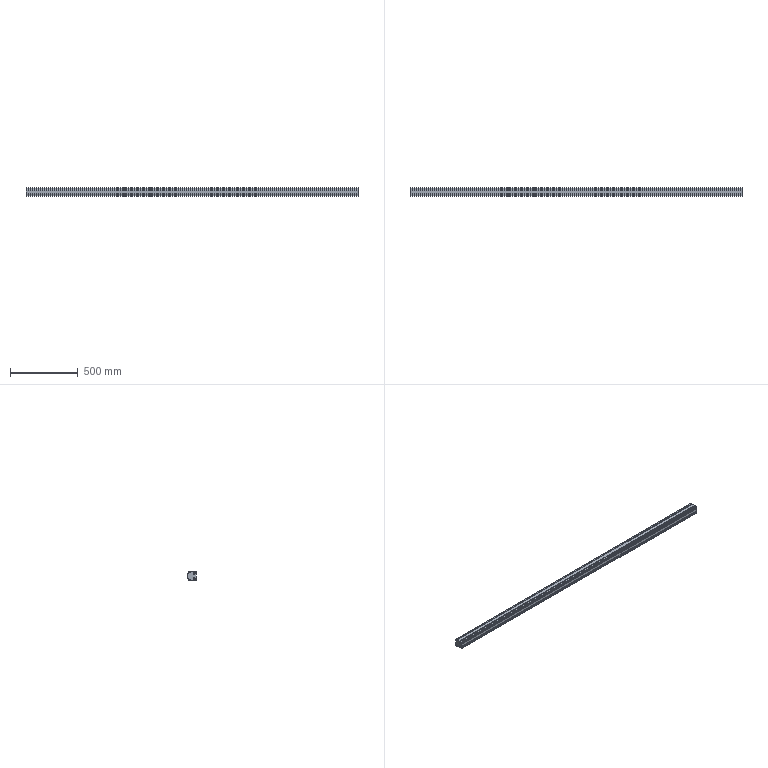Part | STEP file | _Achsprofil-SBG - PAS42 B 1236 | 1 solid | 186 faces | box 2456 x 60 x 60 mm | volume 8161158 mm3 | cylinder 84 | plane 70 | cone 32 | commonest cylinder face diameters 0.4 x22 1 x18 3.242 x16 0.6 x8 6 x8 1.6 x7